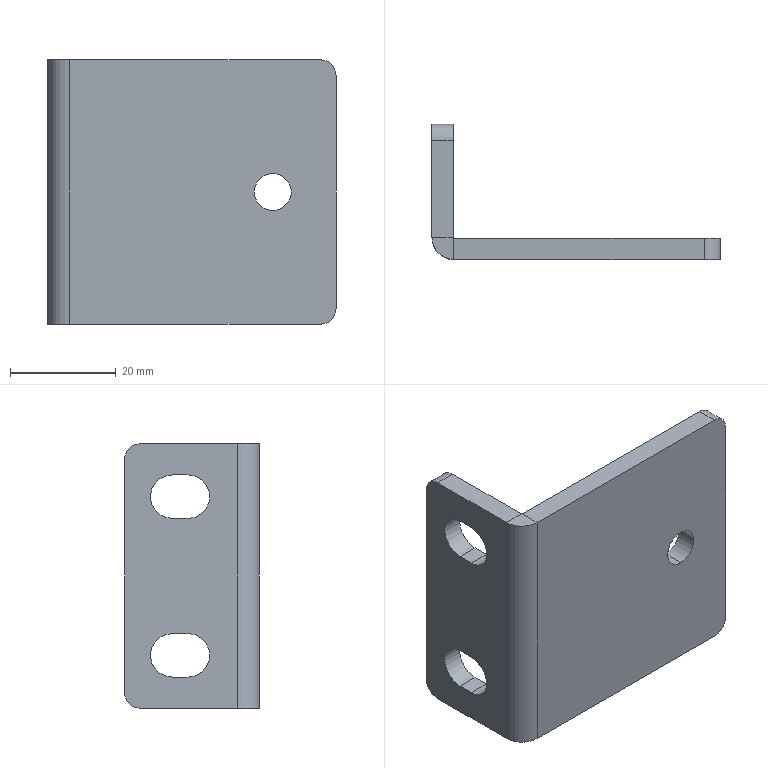Part | STEP file | drive wheel fixing plate | 1 solid | 30 faces | box 54.501 x 25.501 x 50 mm | volume 14216 mm3 | plane 16 | cylinder 14 | commonest cylinder face diameters 8.2 x7 6 x4 7 x2 0.2 x1